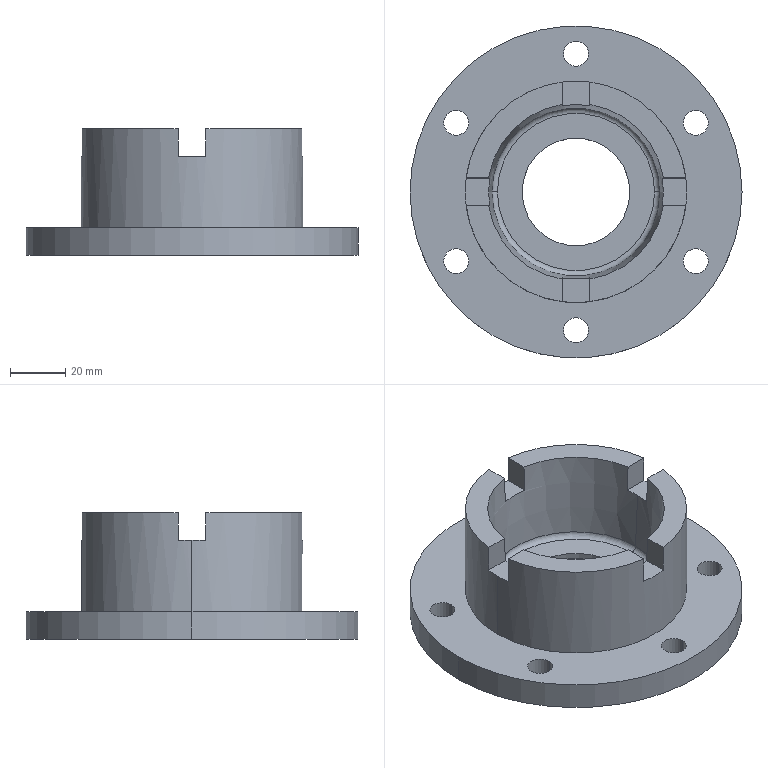Part | SolidWorks | features ICE 6, CirPattern 2, Fillet 1, MirrorPattern 1, RevCut 1, Revolution 1 | 1 solid | 952 faces | box 120 x 120 x 45.75 mm | volume 157075 mm3 | plane 680 | spline 240 | cylinder 22 | cone 6 | torus 4 | commonest cylinder face diameters 9 x12 39 x4 51 x2 80 x2 120 x2